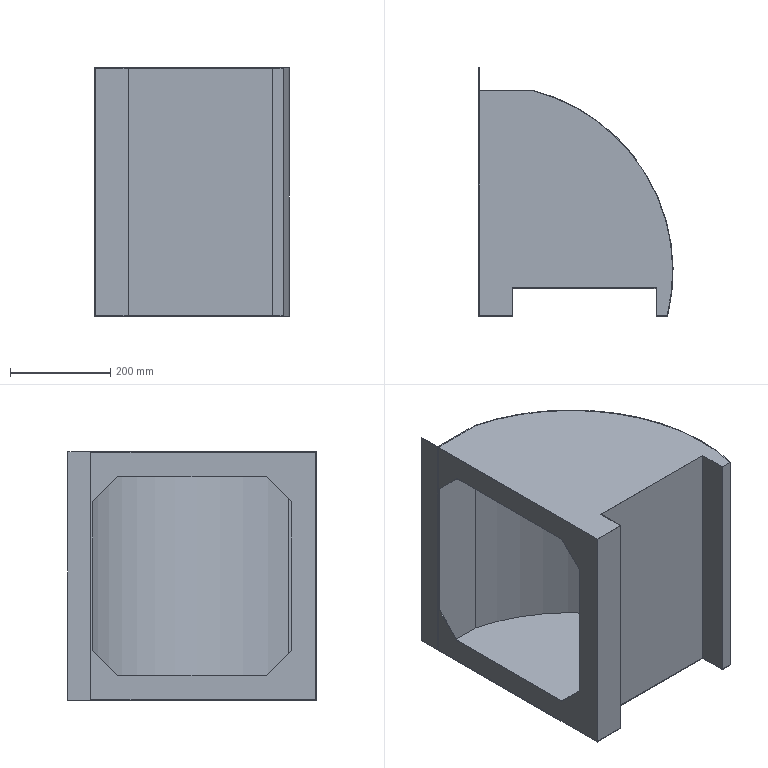Part | SolidWorks | features Extrusion 1, ICE 1, Shell 1 | 1 solid | 33 faces | box 386.98 x 495 x 495.029 mm | volume 841462 mm3 | plane 31 | cylinder 2 | commonest cylinder face diameters 740.359 x1 742.159 x1
STEP:
#1=CARTESIAN_POINT('',(0.,480.,495.));
#2=VERTEX_POINT('',#1);
#3=CARTESIAN_POINT('',(0.,480.,494.971));
#4=VERTEX_POINT('',#3);
#5=CARTESIAN_POINT('',(0.,480.,495.));
#6=DIRECTION('',(0.,0.,-1.));
#7=VECTOR('',#6,1000.);
#8=LINE('',#5,#7);
#9=EDGE_CURVE('',#2,#4,#8,.T.);
#10=ORIENTED_EDGE('',*,*,#9,.T.);
#11=CARTESIAN_POINT('',(0.,495.,494.971));
#12=VERTEX_POINT('',#11);
#13=CARTESIAN_POINT('',(0.,0.,494.971));
#14=DIRECTION('',(0.,1.,0.));
#15=VECTOR('',#14,1000.);
#16=LINE('',#13,#15);
#17=EDGE_CURVE('',#4,#12,#16,.T.);
#18=ORIENTED_EDGE('',*,*,#17,.T.);
#19=CARTESIAN_POINT('',(0.,495.,-0.02854));
#20=VERTEX_POINT('',#19);
#21=CARTESIAN_POINT('',(0.,495.,0.));
#22=DIRECTION('',(0.,0.,-1.));
#23=VECTOR('',#22,1000.);
#24=LINE('',#21,#23);
#25=EDGE_CURVE('',#12,#20,#24,.T.);
#26=ORIENTED_EDGE('',*,*,#25,.T.);
#27=CARTESIAN_POINT('',(0.,0.,-0.02854));
#28=VERTEX_POINT('',#27);
#29=CARTESIAN_POINT('',(0.,0.,-0.02854));
#30=DIRECTION('',(0.,-1.,0.));
#31=VECTOR('',#30,1000.);
#32=LINE('',#29,#31);
#33=EDGE_CURVE('',#20,#28,#32,.T.);
#34=ORIENTED_EDGE('',*,*,#33,.T.);
#35=CARTESIAN_POINT('',(0.,0.,495.));
#36=VERTEX_POINT('',#35);
#37=CARTESIAN_POINT('',(0.,0.,495.));
#38=DIRECTION('',(0.,0.,-1.));
#39=VECTOR('',#38,1000.);
#40=LINE('',#37,#39);
#41=EDGE_CURVE('',#36,#28,#40,.T.);
#42=ORIENTED_EDGE('',*,*,#41,.F.);
#43=CARTESIAN_POINT('',(0.,450.,495.));
#44=DIRECTION('',(0.,-1.,0.));
#45=VECTOR('',#44,1000.);
#46=LINE('',#43,#45);
#47=EDGE_CURVE('',#2,#36,#46,.T.);
#48=ORIENTED_EDGE('',*,*,#47,.F.);
#49=EDGE_LOOP('',(#10,#18,#26,#34,#42,#48));
#50=FACE_OUTER_BOUND('',#49,.T.);
#51=CARTESIAN_POINT('',(0.,50.,394.971));
#52=VERTEX_POINT('',#51);
#53=CARTESIAN_POINT('',(0.,100.,444.971));
#54=VERTEX_POINT('',#53);
#55=CARTESIAN_POINT('',(0.,-172.486,172.486));
#56=DIRECTION('',(0.,0.7071,0.7071));
#57=VECTOR('',#56,1000.);
#58=LINE('',#55,#57);
#59=EDGE_CURVE('',#52,#54,#58,.T.);
#60=ORIENTED_EDGE('',*,*,#59,.F.);
#61=CARTESIAN_POINT('',(0.,50.,99.971));
#62=VERTEX_POINT('',#61);
#63=CARTESIAN_POINT('',(0.,50.,0.));
#64=DIRECTION('',(0.,0.,1.));
#65=VECTOR('',#64,1000.);
#66=LINE('',#63,#65);
#67=EDGE_CURVE('',#62,#52,#66,.T.);
#68=ORIENTED_EDGE('',*,*,#67,.F.);
#69=CARTESIAN_POINT('',(0.,100.,49.971));
#70=VERTEX_POINT('',#69);
#71=CARTESIAN_POINT('',(0.,74.986,74.986));
#72=DIRECTION('',(0.,0.7071,-0.7071));
#73=VECTOR('',#72,1000.);
#74=LINE('',#71,#73);
#75=EDGE_CURVE('',#62,#70,#74,.T.);
#76=ORIENTED_EDGE('',*,*,#75,.T.);
#77=CARTESIAN_POINT('',(0.,395.,49.971));
#78=VERTEX_POINT('',#77);
#79=CARTESIAN_POINT('',(0.,0.,49.971));
#80=DIRECTION('',(0.,-1.,0.));
#81=VECTOR('',#80,1000.);
#82=LINE('',#79,#81);
#83=EDGE_CURVE('',#78,#70,#82,.T.);
#84=ORIENTED_EDGE('',*,*,#83,.F.);
#85=CARTESIAN_POINT('',(0.,445.,99.971));
#86=VERTEX_POINT('',#85);
#87=CARTESIAN_POINT('',(0.,172.514,-172.514));
#88=DIRECTION('',(0.,-0.7071,-0.7071));
#89=VECTOR('',#88,1000.);
#90=LINE('',#87,#89);
#91=EDGE_CURVE('',#86,#78,#90,.T.);
#92=ORIENTED_EDGE('',*,*,#91,.F.);
#93=CARTESIAN_POINT('',(0.,445.,394.971));
#94=VERTEX_POINT('',#93);
#95=CARTESIAN_POINT('',(0.,445.,0.));
#96=DIRECTION('',(0.,0.,-1.));
#97=VECTOR('',#96,1000.);
#98=LINE('',#95,#97);
#99=EDGE_CURVE('',#94,#86,#98,.T.);
#100=ORIENTED_EDGE('',*,*,#99,.F.);
#101=CARTESIAN_POINT('',(0.,395.,444.971));
#102=VERTEX_POINT('',#101);
#103=CARTESIAN_POINT('',(0.,419.986,419.986));
#104=DIRECTION('',(0.,-0.7071,0.7071));
#105=VECTOR('',#104,1000.);
#106=LINE('',#103,#105);
#107=EDGE_CURVE('',#94,#102,#106,.T.);
#108=ORIENTED_EDGE('',*,*,#107,.T.);
#109=CARTESIAN_POINT('',(0.,0.,444.971));
#110=DIRECTION('',(0.,1.,0.));
#111=VECTOR('',#110,1000.);
#112=LINE('',#109,#111);
#113=EDGE_CURVE('',#54,#102,#112,.T.);
#114=ORIENTED_EDGE('',*,*,#113,.F.);
#115=EDGE_LOOP('',(#60,#68,#76,#84,#92,#100,#108,#114));
#116=FACE_BOUND('',#115,.T.);
#117=CARTESIAN_POINT('',(0.,450.,495.));
#118=DIRECTION('',(1.,0.,0.));
#119=DIRECTION('',(0.,0.,-1.));
#120=AXIS2_PLACEMENT_3D('',#117,#118,#119);
#121=PLANE('',#120);
#122=ADVANCED_FACE('',(#50,#116),#121,.F.);
#123=ORIENTED_EDGE('',*,*,#41,.T.);
#124=CARTESIAN_POINT('',(0.9,0.,-0.02854));
#125=VERTEX_POINT('',#124);
#126=CARTESIAN_POINT('',(0.9,0.,-0.02854));
#127=DIRECTION('',(-1.,0.,0.));
#128=VECTOR('',#127,1000.);
#129=LINE('',#126,#128);
#130=EDGE_CURVE('',#125,#28,#129,.T.);
#131=ORIENTED_EDGE('',*,*,#130,.F.);
#132=CARTESIAN_POINT('',(0.9,0.,0.));
#133=VERTEX_POINT('',#132);
#134=CARTESIAN_POINT('',(0.9,0.,0.));
#135=DIRECTION('',(0.,0.,1.));
#136=VECTOR('',#135,1000.);
#137=LINE('',#134,#136);
#138=EDGE_CURVE('',#125,#133,#137,.T.);
#139=ORIENTED_EDGE('',*,*,#138,.T.);
#140=CARTESIAN_POINT('',(67.,0.,0.));
#141=VERTEX_POINT('',#140);
#142=CARTESIAN_POINT('',(0.,0.,0.));
#143=DIRECTION('',(1.,0.,0.));
#144=VECTOR('',#143,1000.);
#145=LINE('',#142,#144);
#146=EDGE_CURVE('',#133,#141,#145,.T.);
#147=ORIENTED_EDGE('',*,*,#146,.T.);
#148=CARTESIAN_POINT('',(67.,0.,495.));
#149=VERTEX_POINT('',#148);
#150=CARTESIAN_POINT('',(67.,0.,495.));
#151=DIRECTION('',(0.,0.,-1.));
#152=VECTOR('',#151,1000.);
#153=LINE('',#150,#152);
#154=EDGE_CURVE('',#149,#141,#153,.T.);
#155=ORIENTED_EDGE('',*,*,#154,.F.);
#156=CARTESIAN_POINT('',(0.,0.,495.));
#157=DIRECTION('',(1.,0.,0.));
#158=VECTOR('',#157,1000.);
#159=LINE('',#156,#158);
#160=EDGE_CURVE('',#36,#149,#159,.T.);
#161=ORIENTED_EDGE('',*,*,#160,.F.);
#162=EDGE_LOOP('',(#123,#131,#139,#147,#155,#161));
#163=FACE_OUTER_BOUND('',#162,.T.);
#164=CARTESIAN_POINT('',(0.,0.,495.));
#165=DIRECTION('',(0.,1.,0.));
#166=DIRECTION('',(0.,0.,1.));
#167=AXIS2_PLACEMENT_3D('',#164,#165,#166);
#168=PLANE('',#167);
#169=ADVANCED_FACE('',(#163),#168,.F.);
#170=CARTESIAN_POINT('',(67.,55.18,0.));
#171=VERTEX_POINT('',#170);
#172=CARTESIAN_POINT('',(67.,0.,0.));
#173=DIRECTION('',(0.,1.,0.));
#174=VECTOR('',#173,1000.);
#175=LINE('',#172,#174);
#176=EDGE_CURVE('',#141,#171,#175,.T.);
#177=ORIENTED_EDGE('',*,*,#176,.T.);
#178=CARTESIAN_POINT('',(67.,55.18,495.));
#179=VERTEX_POINT('',#178);
#180=CARTESIAN_POINT('',(67.,55.18,495.));
#181=DIRECTION('',(0.,0.,-1.));
#182=VECTOR('',#181,1000.);
#183=LINE('',#180,#182);
#184=EDGE_CURVE('',#179,#171,#183,.T.);
#185=ORIENTED_EDGE('',*,*,#184,.F.);
#186=CARTESIAN_POINT('',(67.,0.,495.));
#187=DIRECTION('',(0.,1.,0.));
#188=VECTOR('',#187,1000.);
#189=LINE('',#186,#188);
#190=EDGE_CURVE('',#149,#179,#189,.T.);
#191=ORIENTED_EDGE('',*,*,#190,.F.);
#192=ORIENTED_EDGE('',*,*,#154,.T.);
#193=EDGE_LOOP('',(#177,#185,#191,#192));
#194=FACE_OUTER_BOUND('',#193,.T.);
#195=CARTESIAN_POINT('',(67.,0.,495.));
#196=DIRECTION('',(-1.,0.,0.));
#197=DIRECTION('',(0.,0.,1.));
#198=AXIS2_PLACEMENT_3D('',#195,#196,#197);
#199=PLANE('',#198);
#200=ADVANCED_FACE('',(#194),#199,.F.);
#201=CARTESIAN_POINT('',(352.9,55.18,0.));
#202=VERTEX_POINT('',#201);
#203=CARTESIAN_POINT('',(67.,55.18,0.));
#204=DIRECTION('',(1.,0.,0.));
#205=VECTOR('',#204,1000.);
#206=LINE('',#203,#205);
#207=EDGE_CURVE('',#171,#202,#206,.T.);
#208=ORIENTED_EDGE('',*,*,#207,.T.);
#209=CARTESIAN_POINT('',(352.9,55.18,495.));
#210=VERTEX_POINT('',#209);
#211=CARTESIAN_POINT('',(352.9,55.18,495.));
#212=DIRECTION('',(0.,0.,-1.));
#213=VECTOR('',#212,1000.);
#214=LINE('',#211,#213);
#215=EDGE_CURVE('',#210,#202,#214,.T.);
#216=ORIENTED_EDGE('',*,*,#215,.F.);
#217=CARTESIAN_POINT('',(67.,55.18,495.));
#218=DIRECTION('',(1.,0.,0.));
#219=VECTOR('',#218,1000.);
#220=LINE('',#217,#219);
#221=EDGE_CURVE('',#179,#210,#220,.T.);
#222=ORIENTED_EDGE('',*,*,#221,.F.);
#223=ORIENTED_EDGE('',*,*,#184,.T.);
#224=EDGE_LOOP('',(#208,#216,#222,#223));
#225=FACE_OUTER_BOUND('',#224,.T.);
#226=CARTESIAN_POINT('',(67.,55.18,495.));
#227=DIRECTION('',(0.,1.,0.));
#228=DIRECTION('',(0.,0.,1.));
#229=AXIS2_PLACEMENT_3D('',#226,#227,#228);
#230=PLANE('',#229);
#231=ADVANCED_FACE('',(#225),#230,.F.);
#232=CARTESIAN_POINT('',(352.9,0.,0.));
#233=VERTEX_POINT('',#232);
#234=CARTESIAN_POINT('',(352.9,55.18,0.));
#235=DIRECTION('',(0.,-1.,0.));
#236=VECTOR('',#235,1000.);
#237=LINE('',#234,#236);
#238=EDGE_CURVE('',#202,#233,#237,.T.);
#239=ORIENTED_EDGE('',*,*,#238,.T.);
#240=CARTESIAN_POINT('',(352.9,0.,495.));
#241=VERTEX_POINT('',#240);
#242=CARTESIAN_POINT('',(352.9,0.,495.));
#243=DIRECTION('',(0.,0.,-1.));
#244=VECTOR('',#243,1000.);
#245=LINE('',#242,#244);
#246=EDGE_CURVE('',#241,#233,#245,.T.);
#247=ORIENTED_EDGE('',*,*,#246,.F.);
#248=CARTESIAN_POINT('',(352.9,55.18,495.));
#249=DIRECTION('',(0.,-1.,0.));
#250=VECTOR('',#249,1000.);
#251=LINE('',#248,#250);
#252=EDGE_CURVE('',#210,#241,#251,.T.);
#253=ORIENTED_EDGE('',*,*,#252,.F.);
#254=ORIENTED_EDGE('',*,*,#215,.T.);
#255=EDGE_LOOP('',(#239,#247,#253,#254));
#256=FACE_OUTER_BOUND('',#255,.T.);
#257=CARTESIAN_POINT('',(352.9,55.18,495.));
#258=DIRECTION('',(1.,0.,0.));
#259=DIRECTION('',(0.,0.,-1.));
#260=AXIS2_PLACEMENT_3D('',#257,#258,#259);
#261=PLANE('',#260);
#262=ADVANCED_FACE('',(#256),#261,.F.);
#263=CARTESIAN_POINT('',(375.9,0.,0.));
#264=VERTEX_POINT('',#263);
#265=CARTESIAN_POINT('',(352.9,0.,0.));
#266=DIRECTION('',(1.,0.,0.));
#267=VECTOR('',#266,1000.);
#268=LINE('',#265,#267);
#269=EDGE_CURVE('',#233,#264,#268,.T.);
#270=ORIENTED_EDGE('',*,*,#269,.T.);
#271=CARTESIAN_POINT('',(375.9,0.,495.));
#272=VERTEX_POINT('',#271);
#273=CARTESIAN_POINT('',(375.9,0.,495.));
#274=DIRECTION('',(0.,0.,-1.));
#275=VECTOR('',#274,1000.);
#276=LINE('',#273,#275);
#277=EDGE_CURVE('',#272,#264,#276,.T.);
#278=ORIENTED_EDGE('',*,*,#277,.F.);
#279=CARTESIAN_POINT('',(352.9,0.,495.));
#280=DIRECTION('',(1.,0.,0.));
#281=VECTOR('',#280,1000.);
#282=LINE('',#279,#281);
#283=EDGE_CURVE('',#241,#272,#282,.T.);
#284=ORIENTED_EDGE('',*,*,#283,.F.);
#285=ORIENTED_EDGE('',*,*,#246,.T.);
#286=EDGE_LOOP('',(#270,#278,#284,#285));
#287=FACE_OUTER_BOUND('',#286,.T.);
#288=CARTESIAN_POINT('',(352.9,0.,495.));
#289=DIRECTION('',(0.,1.,0.));
#290=DIRECTION('',(0.,0.,1.));
#291=AXIS2_PLACEMENT_3D('',#288,#289,#290);
#292=PLANE('',#291);
#293=ADVANCED_FACE('',(#287),#292,.F.);
#294=CARTESIAN_POINT('',(105.9,450.,0.));
#295=VERTEX_POINT('',#294);
#296=CARTESIAN_POINT('',(15.9,90.,0.));
#297=DIRECTION('',(0.,0.,1.));
#298=DIRECTION('',(-1.,0.,0.));
#299=AXIS2_PLACEMENT_3D('',#296,#297,#298);
#300=CIRCLE('',#299,371.08);
#301=EDGE_CURVE('',#264,#295,#300,.T.);
#302=ORIENTED_EDGE('',*,*,#301,.T.);
#303=CARTESIAN_POINT('',(105.9,450.,495.));
#304=VERTEX_POINT('',#303);
#305=CARTESIAN_POINT('',(105.9,450.,495.));
#306=DIRECTION('',(0.,0.,-1.));
#307=VECTOR('',#306,1000.);
#308=LINE('',#305,#307);
#309=EDGE_CURVE('',#304,#295,#308,.T.);
#310=ORIENTED_EDGE('',*,*,#309,.F.);
#311=CARTESIAN_POINT('',(15.9,90.,495.));
#312=DIRECTION('',(0.,0.,1.));
#313=DIRECTION('',(-1.,0.,0.));
#314=AXIS2_PLACEMENT_3D('',#311,#312,#313);
#315=CIRCLE('',#314,371.08);
#316=EDGE_CURVE('',#272,#304,#315,.T.);
#317=ORIENTED_EDGE('',*,*,#316,.F.);
#318=ORIENTED_EDGE('',*,*,#277,.T.);
#319=EDGE_LOOP('',(#302,#310,#317,#318));
#320=FACE_OUTER_BOUND('',#319,.T.);
#321=CARTESIAN_POINT('',(15.9,90.,495.));
#322=DIRECTION('',(0.,0.,-1.));
#323=DIRECTION('',(-1.,0.,0.));
#324=AXIS2_PLACEMENT_3D('',#321,#322,#323);
#325=CYLINDRICAL_SURFACE('',#324,371.08);
#326=ADVANCED_FACE('',(#320),#325,.T.);
#327=CARTESIAN_POINT('',(0.9,450.,0.));
#328=VERTEX_POINT('',#327);
#329=CARTESIAN_POINT('',(0.9,450.,0.));
#330=DIRECTION('',(-1.,0.,0.));
#331=VECTOR('',#330,1000.);
#332=LINE('',#329,#331);
#333=EDGE_CURVE('',#295,#328,#332,.T.);
#334=ORIENTED_EDGE('',*,*,#333,.T.);
#335=CARTESIAN_POINT('',(0.9,450.,495.));
#336=VERTEX_POINT('',#335);
#337=CARTESIAN_POINT('',(0.9,450.,495.));
#338=DIRECTION('',(0.,0.,-1.));
#339=VECTOR('',#338,1000.);
#340=LINE('',#337,#339);
#341=EDGE_CURVE('',#336,#328,#340,.T.);
#342=ORIENTED_EDGE('',*,*,#341,.F.);
#343=CARTESIAN_POINT('',(0.9,450.,495.));
#344=DIRECTION('',(-1.,0.,0.));
#345=VECTOR('',#344,1000.);
#346=LINE('',#343,#345);
#347=EDGE_CURVE('',#304,#336,#346,.T.);
#348=ORIENTED_EDGE('',*,*,#347,.F.);
#349=ORIENTED_EDGE('',*,*,#309,.T.);
#350=EDGE_LOOP('',(#334,#342,#348,#349));
#351=FACE_OUTER_BOUND('',#350,.T.);
#352=CARTESIAN_POINT('',(0.9,450.,495.));
#353=DIRECTION('',(0.,-1.,0.));
#354=DIRECTION('',(0.,0.,-1.));
#355=AXIS2_PLACEMENT_3D('',#352,#353,#354);
#356=PLANE('',#355);
#357=ADVANCED_FACE('',(#351),#356,.F.);
#358=ORIENTED_EDGE('',*,*,#341,.T.);
#359=CARTESIAN_POINT('',(0.9,90.,0.));
#360=DIRECTION('',(0.,-1.,0.));
#361=VECTOR('',#360,1000.);
#362=LINE('',#359,#361);
#363=EDGE_CURVE('',#328,#133,#362,.T.);
#364=ORIENTED_EDGE('',*,*,#363,.T.);
#365=ORIENTED_EDGE('',*,*,#138,.F.);
#366=CARTESIAN_POINT('',(0.9,495.,-0.02854));
#367=VERTEX_POINT('',#366);
#368=CARTESIAN_POINT('',(0.9,0.,-0.02854));
#369=DIRECTION('',(0.,-1.,0.));
#370=VECTOR('',#369,1000.);
#371=LINE('',#368,#370);
#372=EDGE_CURVE('',#367,#125,#371,.T.);
#373=ORIENTED_EDGE('',*,*,#372,.F.);
#374=CARTESIAN_POINT('',(0.9,495.,494.971));
#375=VERTEX_POINT('',#374);
#376=CARTESIAN_POINT('',(0.9,495.,0.));
#377=DIRECTION('',(0.,0.,-1.));
#378=VECTOR('',#377,1000.);
#379=LINE('',#376,#378);
#380=EDGE_CURVE('',#375,#367,#379,.T.);
#381=ORIENTED_EDGE('',*,*,#380,.F.);
#382=CARTESIAN_POINT('',(0.9,480.,494.971));
#383=VERTEX_POINT('',#382);
#384=CARTESIAN_POINT('',(0.9,0.,494.971));
#385=DIRECTION('',(0.,1.,0.));
#386=VECTOR('',#385,1000.);
#387=LINE('',#384,#386);
#388=EDGE_CURVE('',#383,#375,#387,.T.);
#389=ORIENTED_EDGE('',*,*,#388,.F.);
#390=CARTESIAN_POINT('',(0.9,480.,495.));
#391=VERTEX_POINT('',#390);
#392=CARTESIAN_POINT('',(0.9,480.,495.));
#393=DIRECTION('',(0.,0.,-1.));
#394=VECTOR('',#393,1000.);
#395=LINE('',#392,#394);
#396=EDGE_CURVE('',#391,#383,#395,.T.);
#397=ORIENTED_EDGE('',*,*,#396,.F.);
#398=CARTESIAN_POINT('',(0.9,480.,495.));
#399=DIRECTION('',(0.,1.,0.));
#400=VECTOR('',#399,1000.);
#401=LINE('',#398,#400);
#402=EDGE_CURVE('',#336,#391,#401,.T.);
#403=ORIENTED_EDGE('',*,*,#402,.F.);
#404=EDGE_LOOP('',(#358,#364,#365,#373,#381,#389,#397,#403));
#405=FACE_OUTER_BOUND('',#404,.T.);
#406=CARTESIAN_POINT('',(0.9,480.,495.));
#407=DIRECTION('',(-1.,0.,0.));
#408=DIRECTION('',(0.,-1.,0.));
#409=AXIS2_PLACEMENT_3D('',#406,#407,#408);
#410=PLANE('',#409);
#411=ADVANCED_FACE('',(#405),#410,.F.);
#412=ORIENTED_EDGE('',*,*,#396,.T.);
#413=CARTESIAN_POINT('',(0.,480.,494.971));
#414=DIRECTION('',(-1.,0.,0.));
#415=VECTOR('',#414,1000.);
#416=LINE('',#413,#415);
#417=EDGE_CURVE('',#383,#4,#416,.T.);
#418=ORIENTED_EDGE('',*,*,#417,.T.);
#419=ORIENTED_EDGE('',*,*,#9,.F.);
#420=CARTESIAN_POINT('',(0.,480.,495.));
#421=DIRECTION('',(-1.,0.,0.));
#422=VECTOR('',#421,1000.);
#423=LINE('',#420,#422);
#424=EDGE_CURVE('',#391,#2,#423,.T.);
#425=ORIENTED_EDGE('',*,*,#424,.F.);
#426=EDGE_LOOP('',(#412,#418,#419,#425));
#427=FACE_OUTER_BOUND('',#426,.T.);
#428=CARTESIAN_POINT('',(0.,480.,495.));
#429=DIRECTION('',(0.,-1.,0.));
#430=DIRECTION('',(0.,0.,-1.));
#431=AXIS2_PLACEMENT_3D('',#428,#429,#430);
#432=PLANE('',#431);
#433=ADVANCED_FACE('',(#427),#432,.F.);
#434=ORIENTED_EDGE('',*,*,#47,.T.);
#435=ORIENTED_EDGE('',*,*,#160,.T.);
#436=ORIENTED_EDGE('',*,*,#190,.T.);
#437=ORIENTED_EDGE('',*,*,#221,.T.);
#438=ORIENTED_EDGE('',*,*,#252,.T.);
#439=ORIENTED_EDGE('',*,*,#283,.T.);
#440=ORIENTED_EDGE('',*,*,#316,.T.);
#441=ORIENTED_EDGE('',*,*,#347,.T.);
#442=ORIENTED_EDGE('',*,*,#402,.T.);
#443=ORIENTED_EDGE('',*,*,#424,.T.);
#444=EDGE_LOOP('',(#434,#435,#436,#437,#438,#439,#440,#441,#442,#443));
#445=FACE_OUTER_BOUND('',#444,.T.);
#446=CARTESIAN_POINT('',(15.9,90.,495.));
#447=DIRECTION('',(0.,0.,-1.));
#448=DIRECTION('',(-1.,0.,0.));
#449=AXIS2_PLACEMENT_3D('',#446,#447,#448);
#450=PLANE('',#449);
#451=ADVANCED_FACE('',(#445),#450,.F.);
#452=ORIENTED_EDGE('',*,*,#363,.F.);
#453=ORIENTED_EDGE('',*,*,#333,.F.);
#454=ORIENTED_EDGE('',*,*,#301,.F.);
#455=ORIENTED_EDGE('',*,*,#269,.F.);
#456=ORIENTED_EDGE('',*,*,#238,.F.);
#457=ORIENTED_EDGE('',*,*,#207,.F.);
#458=ORIENTED_EDGE('',*,*,#176,.F.);
#459=ORIENTED_EDGE('',*,*,#146,.F.);
#460=EDGE_LOOP('',(#452,#453,#454,#455,#456,#457,#458,#459));
#461=FACE_OUTER_BOUND('',#460,.T.);
#462=CARTESIAN_POINT('',(15.9,90.,0.));
#463=DIRECTION('',(0.,0.,-1.));
#464=DIRECTION('',(-1.,0.,0.));
#465=AXIS2_PLACEMENT_3D('',#462,#463,#464);
#466=PLANE('',#465);
#467=ADVANCED_FACE('',(#461),#466,.T.);
#468=ORIENTED_EDGE('',*,*,#113,.T.);
#469=CARTESIAN_POINT('',(0.9,395.,444.971));
#470=VERTEX_POINT('',#469);
#471=CARTESIAN_POINT('',(0.9,395.,444.971));
#472=DIRECTION('',(-1.,0.,0.));
#473=VECTOR('',#472,1000.);
#474=LINE('',#471,#473);
#475=EDGE_CURVE('',#470,#102,#474,.T.);
#476=ORIENTED_EDGE('',*,*,#475,.F.);
#477=CARTESIAN_POINT('',(0.9,100.,444.971));
#478=VERTEX_POINT('',#477);
#479=CARTESIAN_POINT('',(0.9,0.,444.971));
#480=DIRECTION('',(0.,1.,0.));
#481=VECTOR('',#480,1000.);
#482=LINE('',#479,#481);
#483=EDGE_CURVE('',#478,#470,#482,.T.);
#484=ORIENTED_EDGE('',*,*,#483,.F.);
#485=CARTESIAN_POINT('',(0.9,100.,444.971));
#486=DIRECTION('',(-1.,0.,0.));
#487=VECTOR('',#486,1000.);
#488=LINE('',#485,#487);
#489=EDGE_CURVE('',#478,#54,#488,.T.);
#490=ORIENTED_EDGE('',*,*,#489,.T.);
#491=EDGE_LOOP('',(#468,#476,#484,#490));
#492=FACE_OUTER_BOUND('',#491,.T.);
#493=CARTESIAN_POINT('',(0.9,0.,444.971));
#494=DIRECTION('',(0.,0.,1.));
#495=DIRECTION('',(1.,0.,0.));
#496=AXIS2_PLACEMENT_3D('',#493,#494,#495);
#497=PLANE('',#496);
#498=ADVANCED_FACE('',(#492),#497,.F.);
#499=ORIENTED_EDGE('',*,*,#107,.F.);
#500=CARTESIAN_POINT('',(0.9,445.,394.971));
#501=VERTEX_POINT('',#500);
#502=CARTESIAN_POINT('',(0.9,445.,394.971));
#503=DIRECTION('',(-1.,0.,0.));
#504=VECTOR('',#503,1000.);
#505=LINE('',#502,#504);
#506=EDGE_CURVE('',#501,#94,#505,.T.);
#507=ORIENTED_EDGE('',*,*,#506,.F.);
#508=CARTESIAN_POINT('',(0.9,419.986,419.986));
#509=DIRECTION('',(0.,-0.7071,0.7071));
#510=VECTOR('',#509,1000.);
#511=LINE('',#508,#510);
#512=EDGE_CURVE('',#501,#470,#511,.T.);
#513=ORIENTED_EDGE('',*,*,#512,.T.);
#514=ORIENTED_EDGE('',*,*,#475,.T.);
#515=EDGE_LOOP('',(#499,#507,#513,#514));
#516=FACE_OUTER_BOUND('',#515,.T.);
#517=CARTESIAN_POINT('',(0.9,419.986,419.986));
#518=DIRECTION('',(0.,-0.7071,-0.7071));
#519=DIRECTION('',(0.,0.7071,-0.7071));
#520=AXIS2_PLACEMENT_3D('',#517,#518,#519);
#521=PLANE('',#520);
#522=ADVANCED_FACE('',(#516),#521,.T.);
#523=ORIENTED_EDGE('',*,*,#99,.T.);
#524=CARTESIAN_POINT('',(0.9,445.,99.971));
#525=VERTEX_POINT('',#524);
#526=CARTESIAN_POINT('',(0.9,445.,99.971));
#527=DIRECTION('',(-1.,0.,0.));
#528=VECTOR('',#527,1000.);
#529=LINE('',#526,#528);
#530=EDGE_CURVE('',#525,#86,#529,.T.);
#531=ORIENTED_EDGE('',*,*,#530,.F.);
#532=CARTESIAN_POINT('',(0.9,445.,0.));
#533=DIRECTION('',(0.,0.,-1.));
#534=VECTOR('',#533,1000.);
#535=LINE('',#532,#534);
#536=EDGE_CURVE('',#501,#525,#535,.T.);
#537=ORIENTED_EDGE('',*,*,#536,.F.);
#538=ORIENTED_EDGE('',*,*,#506,.T.);
#539=EDGE_LOOP('',(#523,#531,#537,#538));
#540=FACE_OUTER_BOUND('',#539,.T.);
#541=CARTESIAN_POINT('',(0.9,445.,0.));
#542=DIRECTION('',(0.,1.,0.));
#543=DIRECTION('',(0.,0.,1.));
#544=AXIS2_PLACEMENT_3D('',#541,#542,#543);
#545=PLANE('',#544);
#546=ADVANCED_FACE('',(#540),#545,.F.);
#547=ORIENTED_EDGE('',*,*,#91,.T.);
#548=CARTESIAN_POINT('',(0.9,395.,49.971));
#549=VERTEX_POINT('',#548);
#550=CARTESIAN_POINT('',(0.9,395.,49.971));
#551=DIRECTION('',(-1.,0.,0.));
#552=VECTOR('',#551,1000.);
#553=LINE('',#550,#552);
#554=EDGE_CURVE('',#549,#78,#553,.T.);
#555=ORIENTED_EDGE('',*,*,#554,.F.);
#556=CARTESIAN_POINT('',(0.9,172.514,-172.514));
#557=DIRECTION('',(0.,-0.7071,-0.7071));
#558=VECTOR('',#557,1000.);
#559=LINE('',#556,#558);
#560=EDGE_CURVE('',#525,#549,#559,.T.);
#561=ORIENTED_EDGE('',*,*,#560,.F.);
#562=ORIENTED_EDGE('',*,*,#530,.T.);
#563=EDGE_LOOP('',(#547,#555,#561,#562));
#564=FACE_OUTER_BOUND('',#563,.T.);
#565=CARTESIAN_POINT('',(0.9,172.514,-172.514));
#566=DIRECTION('',(0.,0.7071,-0.7071));
#567=DIRECTION('',(0.,0.7071,0.7071));
#568=AXIS2_PLACEMENT_3D('',#565,#566,#567);
#569=PLANE('',#568);
#570=ADVANCED_FACE('',(#564),#569,.F.);
#571=ORIENTED_EDGE('',*,*,#83,.T.);
#572=CARTESIAN_POINT('',(0.9,100.,49.971));
#573=VERTEX_POINT('',#572);
#574=CARTESIAN_POINT('',(0.9,100.,49.971));
#575=DIRECTION('',(-1.,0.,0.));
#576=VECTOR('',#575,1000.);
#577=LINE('',#574,#576);
#578=EDGE_CURVE('',#573,#70,#577,.T.);
#579=ORIENTED_EDGE('',*,*,#578,.F.);
#580=CARTESIAN_POINT('',(0.9,0.,49.971));
#581=DIRECTION('',(0.,-1.,0.));
#582=VECTOR('',#581,1000.);
#583=LINE('',#580,#582);
#584=EDGE_CURVE('',#549,#573,#583,.T.);
#585=ORIENTED_EDGE('',*,*,#584,.F.);
#586=ORIENTED_EDGE('',*,*,#554,.T.);
#587=EDGE_LOOP('',(#571,#579,#585,#586));
#588=FACE_OUTER_BOUND('',#587,.T.);
#589=CARTESIAN_POINT('',(0.9,0.,49.971));
#590=DIRECTION('',(0.,0.,-1.));
#591=DIRECTION('',(-1.,0.,0.));
#592=AXIS2_PLACEMENT_3D('',#589,#590,#591);
#593=PLANE('',#592);
#594=ADVANCED_FACE('',(#588),#593,.F.);
#595=ORIENTED_EDGE('',*,*,#75,.F.);
#596=CARTESIAN_POINT('',(0.9,50.,99.971));
#597=VERTEX_POINT('',#596);
#598=CARTESIAN_POINT('',(0.9,50.,99.971));
#599=DIRECTION('',(-1.,0.,0.));
#600=VECTOR('',#599,1000.);
#601=LINE('',#598,#600);
#602=EDGE_CURVE('',#597,#62,#601,.T.);
#603=ORIENTED_EDGE('',*,*,#602,.F.);
#604=CARTESIAN_POINT('',(0.9,74.986,74.986));
#605=DIRECTION('',(0.,0.7071,-0.7071));
#606=VECTOR('',#605,1000.);
#607=LINE('',#604,#606);
#608=EDGE_CURVE('',#597,#573,#607,.T.);
#609=ORIENTED_EDGE('',*,*,#608,.T.);
#610=ORIENTED_EDGE('',*,*,#578,.T.);
#611=EDGE_LOOP('',(#595,#603,#609,#610));
#612=FACE_OUTER_BOUND('',#611,.T.);
#613=CARTESIAN_POINT('',(0.9,74.986,74.986));
#614=DIRECTION('',(0.,0.7071,0.7071));
#615=DIRECTION('',(0.,-0.7071,0.7071));
#616=AXIS2_PLACEMENT_3D('',#613,#614,#615);
#617=PLANE('',#616);
#618=ADVANCED_FACE('',(#612),#617,.T.);
#619=ORIENTED_EDGE('',*,*,#67,.T.);
#620=CARTESIAN_POINT('',(0.9,50.,394.971));
#621=VERTEX_POINT('',#620);
#622=CARTESIAN_POINT('',(0.9,50.,394.971));
#623=DIRECTION('',(-1.,0.,0.));
#624=VECTOR('',#623,1000.);
#625=LINE('',#622,#624);
#626=EDGE_CURVE('',#621,#52,#625,.T.);
#627=ORIENTED_EDGE('',*,*,#626,.F.);
#628=CARTESIAN_POINT('',(0.9,50.,0.));
#629=DIRECTION('',(0.,0.,1.));
#630=VECTOR('',#629,1000.);
#631=LINE('',#628,#630);
#632=EDGE_CURVE('',#597,#621,#631,.T.);
#633=ORIENTED_EDGE('',*,*,#632,.F.);
#634=ORIENTED_EDGE('',*,*,#602,.T.);
#635=EDGE_LOOP('',(#619,#627,#633,#634));
#636=FACE_OUTER_BOUND('',#635,.T.);
#637=CARTESIAN_POINT('',(0.9,50.,0.));
#638=DIRECTION('',(0.,-1.,0.));
#639=DIRECTION('',(0.,0.,-1.));
#640=AXIS2_PLACEMENT_3D('',#637,#638,#639);
#641=PLANE('',#640);
#642=ADVANCED_FACE('',(#636),#641,.F.);
#643=CARTESIAN_POINT('',(0.9,449.1,0.9));
#644=VERTEX_POINT('',#643);
#645=CARTESIAN_POINT('',(0.9,449.1,494.1));
#646=VERTEX_POINT('',#645);
#647=CARTESIAN_POINT('',(0.9,449.1,495.));
#648=DIRECTION('',(0.,0.,1.));
#649=VECTOR('',#648,1000.);
#650=LINE('',#647,#649);
#651=EDGE_CURVE('',#644,#646,#650,.T.);
#652=ORIENTED_EDGE('',*,*,#651,.T.);
#653=CARTESIAN_POINT('',(0.9,0.9,494.1));
#654=VERTEX_POINT('',#653);
#655=CARTESIAN_POINT('',(0.9,90.,494.1));
#656=DIRECTION('',(0.,-1.,0.));
#657=VECTOR('',#656,1000.);
#658=LINE('',#655,#657);
#659=EDGE_CURVE('',#646,#654,#658,.T.);
#660=ORIENTED_EDGE('',*,*,#659,.T.);
#661=CARTESIAN_POINT('',(0.9,0.9,0.9));
#662=VERTEX_POINT('',#661);
#663=CARTESIAN_POINT('',(0.9,0.9,495.));
#664=DIRECTION('',(0.,0.,-1.));
#665=VECTOR('',#664,1000.);
#666=LINE('',#663,#665);
#667=EDGE_CURVE('',#654,#662,#666,.T.);
#668=ORIENTED_EDGE('',*,*,#667,.T.);
#669=CARTESIAN_POINT('',(0.9,90.,0.9));
#670=DIRECTION('',(0.,-1.,0.));
#671=VECTOR('',#670,1000.);
#672=LINE('',#669,#671);
#673=EDGE_CURVE('',#644,#662,#672,.T.);
#674=ORIENTED_EDGE('',*,*,#673,.F.);
#675=EDGE_LOOP('',(#652,#660,#668,#674));
#676=FACE_OUTER_BOUND('',#675,.T.);
#677=CARTESIAN_POINT('',(0.9,-172.486,172.486));
#678=DIRECTION('',(0.,0.7071,0.7071));
#679=VECTOR('',#678,1000.);
#680=LINE('',#677,#679);
#681=EDGE_CURVE('',#621,#478,#680,.T.);
#682=ORIENTED_EDGE('',*,*,#681,.T.);
#683=ORIENTED_EDGE('',*,*,#483,.T.);
#684=ORIENTED_EDGE('',*,*,#512,.F.);
#685=ORIENTED_EDGE('',*,*,#536,.T.);
#686=ORIENTED_EDGE('',*,*,#560,.T.);
#687=ORIENTED_EDGE('',*,*,#584,.T.);
#688=ORIENTED_EDGE('',*,*,#608,.F.);
#689=ORIENTED_EDGE('',*,*,#632,.T.);
#690=EDGE_LOOP('',(#682,#683,#684,#685,#686,#687,#688,#689));
#691=FACE_BOUND('',#690,.T.);
#692=CARTESIAN_POINT('',(0.9,0.,0.));
#693=DIRECTION('',(1.,0.,0.));
#694=DIRECTION('',(0.,0.,-1.));
#695=AXIS2_PLACEMENT_3D('',#692,#693,#694);
#696=PLANE('',#695);
#697=ADVANCED_FACE('',(#676,#691),#696,.T.);
#698=ORIENTED_EDGE('',*,*,#59,.T.);
#699=ORIENTED_EDGE('',*,*,#489,.F.);
#700=ORIENTED_EDGE('',*,*,#681,.F.);
#701=ORIENTED_EDGE('',*,*,#626,.T.);
#702=EDGE_LOOP('',(#698,#699,#700,#701));
#703=FACE_OUTER_BOUND('',#702,.T.);
#704=CARTESIAN_POINT('',(0.9,-172.486,172.486));
#705=DIRECTION('',(0.,-0.7071,0.7071));
#706=DIRECTION('',(0.,-0.7071,-0.7071));
#707=AXIS2_PLACEMENT_3D('',#704,#705,#706);
#708=PLANE('',#707);
#709=ADVANCED_FACE('',(#703),#708,.F.);
#710=CARTESIAN_POINT('',(375.197,0.9,0.9));
#711=VERTEX_POINT('',#710);
#712=CARTESIAN_POINT('',(105.789,449.1,0.9));
#713=VERTEX_POINT('',#712);
#714=CARTESIAN_POINT('',(15.9,90.,0.9));
#715=DIRECTION('',(0.,0.,1.));
#716=DIRECTION('',(-1.,0.,0.));
#717=AXIS2_PLACEMENT_3D('',#714,#715,#716);
#718=CIRCLE('',#717,370.18);
#719=EDGE_CURVE('',#711,#713,#718,.T.);
#720=ORIENTED_EDGE('',*,*,#719,.F.);
#721=CARTESIAN_POINT('',(375.197,0.9,494.1));
#722=VERTEX_POINT('',#721);
#723=CARTESIAN_POINT('',(375.197,0.9,494.1));
#724=DIRECTION('',(0.,0.,-1.));
#725=VECTOR('',#724,1000.);
#726=LINE('',#723,#725);
#727=EDGE_CURVE('',#722,#711,#726,.T.);
#728=ORIENTED_EDGE('',*,*,#727,.F.);
#729=CARTESIAN_POINT('',(105.789,449.1,494.1));
#730=VERTEX_POINT('',#729);
#731=CARTESIAN_POINT('',(15.9,90.,494.1));
#732=DIRECTION('',(0.,0.,1.));
#733=DIRECTION('',(-1.,0.,0.));
#734=AXIS2_PLACEMENT_3D('',#731,#732,#733);
#735=CIRCLE('',#734,370.18);
#736=EDGE_CURVE('',#722,#730,#735,.T.);
#737=ORIENTED_EDGE('',*,*,#736,.T.);
#738=CARTESIAN_POINT('',(105.789,449.1,494.1));
#739=DIRECTION('',(0.,0.,-1.));
#740=VECTOR('',#739,1000.);
#741=LINE('',#738,#740);
#742=EDGE_CURVE('',#730,#713,#741,.T.);
#743=ORIENTED_EDGE('',*,*,#742,.T.);
#744=EDGE_LOOP('',(#720,#728,#737,#743));
#745=FACE_OUTER_BOUND('',#744,.T.);
#746=CARTESIAN_POINT('',(15.9,90.,495.));
#747=DIRECTION('',(0.,0.,-1.));
#748=DIRECTION('',(-1.,0.,0.));
#749=AXIS2_PLACEMENT_3D('',#746,#747,#748);
#750=CYLINDRICAL_SURFACE('',#749,370.18);
#751=ADVANCED_FACE('',(#745),#750,.F.);
#752=CARTESIAN_POINT('',(353.8,0.9,0.9));
#753=VERTEX_POINT('',#752);
#754=CARTESIAN_POINT('',(15.9,0.9,0.9));
#755=DIRECTION('',(1.,0.,0.));
#756=VECTOR('',#755,1000.);
#757=LINE('',#754,#756);
#758=EDGE_CURVE('',#753,#711,#757,.T.);
#759=ORIENTED_EDGE('',*,*,#758,.F.);
#760=CARTESIAN_POINT('',(353.8,0.9,494.1));
#761=VERTEX_POINT('',#760);
#762=CARTESIAN_POINT('',(353.8,0.9,495.));
#763=DIRECTION('',(0.,0.,-1.));
#764=VECTOR('',#763,1000.);
#765=LINE('',#762,#764);
#766=EDGE_CURVE('',#761,#753,#765,.T.);
#767=ORIENTED_EDGE('',*,*,#766,.F.);
#768=CARTESIAN_POINT('',(15.9,0.9,494.1));
#769=DIRECTION('',(1.,0.,0.));
#770=VECTOR('',#769,1000.);
#771=LINE('',#768,#770);
#772=EDGE_CURVE('',#761,#722,#771,.T.);
#773=ORIENTED_EDGE('',*,*,#772,.T.);
#774=ORIENTED_EDGE('',*,*,#727,.T.);
#775=EDGE_LOOP('',(#759,#767,#773,#774));
#776=FACE_OUTER_BOUND('',#775,.T.);
#777=CARTESIAN_POINT('',(352.9,0.9,495.));
#778=DIRECTION('',(0.,1.,0.));
#779=DIRECTION('',(0.,0.,1.));
#780=AXIS2_PLACEMENT_3D('',#777,#778,#779);
#781=PLANE('',#780);
#782=ADVANCED_FACE('',(#776),#781,.T.);
#783=CARTESIAN_POINT('',(353.8,56.08,0.9));
#784=VERTEX_POINT('',#783);
#785=CARTESIAN_POINT('',(353.8,90.,0.9));
#786=DIRECTION('',(0.,-1.,0.));
#787=VECTOR('',#786,1000.);
#788=LINE('',#785,#787);
#789=EDGE_CURVE('',#784,#753,#788,.T.);
#790=ORIENTED_EDGE('',*,*,#789,.F.);
#791=CARTESIAN_POINT('',(353.8,56.08,494.1));
#792=VERTEX_POINT('',#791);
#793=CARTESIAN_POINT('',(353.8,56.08,495.));
#794=DIRECTION('',(0.,0.,-1.));
#795=VECTOR('',#794,1000.);
#796=LINE('',#793,#795);
#797=EDGE_CURVE('',#792,#784,#796,.T.);
#798=ORIENTED_EDGE('',*,*,#797,.F.);
#799=CARTESIAN_POINT('',(353.8,90.,494.1));
#800=DIRECTION('',(0.,-1.,0.));
#801=VECTOR('',#800,1000.);
#802=LINE('',#799,#801);
#803=EDGE_CURVE('',#792,#761,#802,.T.);
#804=ORIENTED_EDGE('',*,*,#803,.T.);
#805=ORIENTED_EDGE('',*,*,#766,.T.);
#806=EDGE_LOOP('',(#790,#798,#804,#805));
#807=FACE_OUTER_BOUND('',#806,.T.);
#808=CARTESIAN_POINT('',(353.8,55.18,495.));
#809=DIRECTION('',(1.,0.,0.));
#810=DIRECTION('',(0.,0.,-1.));
#811=AXIS2_PLACEMENT_3D('',#808,#809,#810);
#812=PLANE('',#811);
#813=ADVANCED_FACE('',(#807),#812,.T.);
#814=CARTESIAN_POINT('',(66.1,56.08,0.9));
#815=VERTEX_POINT('',#814);
#816=CARTESIAN_POINT('',(15.9,56.08,0.9));
#817=DIRECTION('',(1.,0.,0.));
#818=VECTOR('',#817,1000.);
#819=LINE('',#816,#818);
#820=EDGE_CURVE('',#815,#784,#819,.T.);
#821=ORIENTED_EDGE('',*,*,#820,.F.);
#822=CARTESIAN_POINT('',(66.1,56.08,494.1));
#823=VERTEX_POINT('',#822);
#824=CARTESIAN_POINT('',(66.1,56.08,495.));
#825=DIRECTION('',(0.,0.,-1.));
#826=VECTOR('',#825,1000.);
#827=LINE('',#824,#826);
#828=EDGE_CURVE('',#823,#815,#827,.T.);
#829=ORIENTED_EDGE('',*,*,#828,.F.);
#830=CARTESIAN_POINT('',(15.9,56.08,494.1));
#831=DIRECTION('',(1.,0.,0.));
#832=VECTOR('',#831,1000.);
#833=LINE('',#830,#832);
#834=EDGE_CURVE('',#823,#792,#833,.T.);
#835=ORIENTED_EDGE('',*,*,#834,.T.);
#836=ORIENTED_EDGE('',*,*,#797,.T.);
#837=EDGE_LOOP('',(#821,#829,#835,#836));
#838=FACE_OUTER_BOUND('',#837,.T.);
#839=CARTESIAN_POINT('',(67.,56.08,495.));
#840=DIRECTION('',(0.,1.,0.));
#841=DIRECTION('',(0.,0.,1.));
#842=AXIS2_PLACEMENT_3D('',#839,#840,#841);
#843=PLANE('',#842);
#844=ADVANCED_FACE('',(#838),#843,.T.);
#845=CARTESIAN_POINT('',(66.1,0.9,0.9));
#846=VERTEX_POINT('',#845);
#847=CARTESIAN_POINT('',(66.1,90.,0.9));
#848=DIRECTION('',(0.,1.,0.));
#849=VECTOR('',#848,1000.);
#850=LINE('',#847,#849);
#851=EDGE_CURVE('',#846,#815,#850,.T.);
#852=ORIENTED_EDGE('',*,*,#851,.F.);
#853=CARTESIAN_POINT('',(66.1,0.9,494.1));
#854=VERTEX_POINT('',#853);
#855=CARTESIAN_POINT('',(66.1,0.9,495.));
#856=DIRECTION('',(0.,0.,-1.));
#857=VECTOR('',#856,1000.);
#858=LINE('',#855,#857);
#859=EDGE_CURVE('',#854,#846,#858,.T.);
#860=ORIENTED_EDGE('',*,*,#859,.F.);
#861=CARTESIAN_POINT('',(66.1,90.,494.1));
#862=DIRECTION('',(0.,1.,0.));
#863=VECTOR('',#862,1000.);
#864=LINE('',#861,#863);
#865=EDGE_CURVE('',#854,#823,#864,.T.);
#866=ORIENTED_EDGE('',*,*,#865,.T.);
#867=ORIENTED_EDGE('',*,*,#828,.T.);
#868=EDGE_LOOP('',(#852,#860,#866,#867));
#869=FACE_OUTER_BOUND('',#868,.T.);
#870=CARTESIAN_POINT('',(66.1,0.,495.));
#871=DIRECTION('',(-1.,0.,0.));
#872=DIRECTION('',(0.,0.,1.));
#873=AXIS2_PLACEMENT_3D('',#870,#871,#872);
#874=PLANE('',#873);
#875=ADVANCED_FACE('',(#869),#874,.T.);
#876=ORIENTED_EDGE('',*,*,#659,.F.);
#877=CARTESIAN_POINT('',(15.9,449.1,494.1));
#878=DIRECTION('',(-1.,0.,0.));
#879=VECTOR('',#878,1000.);
#880=LINE('',#877,#879);
#881=EDGE_CURVE('',#730,#646,#880,.T.);
#882=ORIENTED_EDGE('',*,*,#881,.F.);
#883=ORIENTED_EDGE('',*,*,#736,.F.);
#884=ORIENTED_EDGE('',*,*,#772,.F.);
#885=ORIENTED_EDGE('',*,*,#803,.F.);
#886=ORIENTED_EDGE('',*,*,#834,.F.);
#887=ORIENTED_EDGE('',*,*,#865,.F.);
#888=CARTESIAN_POINT('',(15.9,0.9,494.1));
#889=DIRECTION('',(1.,0.,0.));
#890=VECTOR('',#889,1000.);
#891=LINE('',#888,#890);
#892=EDGE_CURVE('',#654,#854,#891,.T.);
#893=ORIENTED_EDGE('',*,*,#892,.F.);
#894=EDGE_LOOP('',(#876,#882,#883,#884,#885,#886,#887,#893));
#895=FACE_OUTER_BOUND('',#894,.T.);
#896=CARTESIAN_POINT('',(15.9,90.,494.1));
#897=DIRECTION('',(0.,0.,-1.));
#898=DIRECTION('',(-1.,0.,0.));
#899=AXIS2_PLACEMENT_3D('',#896,#897,#898);
#900=PLANE('',#899);
#901=ADVANCED_FACE('',(#895),#900,.T.);
#902=CARTESIAN_POINT('',(15.9,449.1,0.9));
#903=DIRECTION('',(-1.,0.,0.));
#904=VECTOR('',#903,1000.);
#905=LINE('',#902,#904);
#906=EDGE_CURVE('',#713,#644,#905,.T.);
#907=ORIENTED_EDGE('',*,*,#906,.T.);
#908=ORIENTED_EDGE('',*,*,#673,.T.);
#909=CARTESIAN_POINT('',(15.9,0.9,0.9));
#910=DIRECTION('',(1.,0.,0.));
#911=VECTOR('',#910,1000.);
#912=LINE('',#909,#911);
#913=EDGE_CURVE('',#662,#846,#912,.T.);
#914=ORIENTED_EDGE('',*,*,#913,.T.);
#915=ORIENTED_EDGE('',*,*,#851,.T.);
#916=ORIENTED_EDGE('',*,*,#820,.T.);
#917=ORIENTED_EDGE('',*,*,#789,.T.);
#918=ORIENTED_EDGE('',*,*,#758,.T.);
#919=ORIENTED_EDGE('',*,*,#719,.T.);
#920=EDGE_LOOP('',(#907,#908,#914,#915,#916,#917,#918,#919));
#921=FACE_OUTER_BOUND('',#920,.T.);
#922=CARTESIAN_POINT('',(15.9,90.,0.9));
#923=DIRECTION('',(0.,0.,-1.));
#924=DIRECTION('',(-1.,0.,0.));
#925=AXIS2_PLACEMENT_3D('',#922,#923,#924);
#926=PLANE('',#925);
#927=ADVANCED_FACE('',(#921),#926,.F.);
#928=ORIENTED_EDGE('',*,*,#651,.F.);
#929=ORIENTED_EDGE('',*,*,#906,.F.);
#930=ORIENTED_EDGE('',*,*,#742,.F.);
#931=ORIENTED_EDGE('',*,*,#881,.T.);
#932=EDGE_LOOP('',(#928,#929,#930,#931));
#933=FACE_OUTER_BOUND('',#932,.T.);
#934=CARTESIAN_POINT('',(0.9,449.1,495.));
#935=DIRECTION('',(0.,-1.,0.));
#936=DIRECTION('',(0.,0.,-1.));
#937=AXIS2_PLACEMENT_3D('',#934,#935,#936);
#938=PLANE('',#937);
#939=ADVANCED_FACE('',(#933),#938,.T.);
#940=ORIENTED_EDGE('',*,*,#667,.F.);
#941=ORIENTED_EDGE('',*,*,#892,.T.);
#942=ORIENTED_EDGE('',*,*,#859,.T.);
#943=ORIENTED_EDGE('',*,*,#913,.F.);
#944=EDGE_LOOP('',(#940,#941,#942,#943));
#945=FACE_OUTER_BOUND('',#944,.T.);
#946=CARTESIAN_POINT('',(0.,0.9,495.));
#947=DIRECTION('',(0.,1.,0.));
#948=DIRECTION('',(0.,0.,1.));
#949=AXIS2_PLACEMENT_3D('',#946,#947,#948);
#950=PLANE('',#949);
#951=ADVANCED_FACE('',(#945),#950,.T.);
#952=ORIENTED_EDGE('',*,*,#417,.F.);
#953=ORIENTED_EDGE('',*,*,#388,.T.);
#954=CARTESIAN_POINT('',(0.9,495.,494.971));
#955=DIRECTION('',(-1.,0.,0.));
#956=VECTOR('',#955,1000.);
#957=LINE('',#954,#956);
#958=EDGE_CURVE('',#375,#12,#957,.T.);
#959=ORIENTED_EDGE('',*,*,#958,.T.);
#960=ORIENTED_EDGE('',*,*,#17,.F.);
#961=EDGE_LOOP('',(#952,#953,#959,#960));
#962=FACE_OUTER_BOUND('',#961,.T.);
#963=CARTESIAN_POINT('',(0.9,0.,494.971));
#964=DIRECTION('',(0.,0.,1.));
#965=DIRECTION('',(1.,0.,0.));
#966=AXIS2_PLACEMENT_3D('',#963,#964,#965);
#967=PLANE('',#966);
#968=ADVANCED_FACE('',(#962),#967,.T.);
#969=ORIENTED_EDGE('',*,*,#33,.F.);
#970=CARTESIAN_POINT('',(0.9,495.,-0.02854));
#971=DIRECTION('',(-1.,0.,0.));
#972=VECTOR('',#971,1000.);
#973=LINE('',#970,#972);
#974=EDGE_CURVE('',#367,#20,#973,.T.);
#975=ORIENTED_EDGE('',*,*,#974,.F.);
#976=ORIENTED_EDGE('',*,*,#372,.T.);
#977=ORIENTED_EDGE('',*,*,#130,.T.);
#978=EDGE_LOOP('',(#969,#975,#976,#977));
#979=FACE_OUTER_BOUND('',#978,.T.);
#980=CARTESIAN_POINT('',(0.9,0.,-0.02854));
#981=DIRECTION('',(0.,0.,-1.));
#982=DIRECTION('',(-1.,0.,0.));
#983=AXIS2_PLACEMENT_3D('',#980,#981,#982);
#984=PLANE('',#983);
#985=ADVANCED_FACE('',(#979),#984,.T.);
#986=ORIENTED_EDGE('',*,*,#25,.F.);
#987=ORIENTED_EDGE('',*,*,#958,.F.);
#988=ORIENTED_EDGE('',*,*,#380,.T.);
#989=ORIENTED_EDGE('',*,*,#974,.T.);
#990=EDGE_LOOP('',(#986,#987,#988,#989));
#991=FACE_OUTER_BOUND('',#990,.T.);
#992=CARTESIAN_POINT('',(0.9,495.,0.));
#993=DIRECTION('',(0.,1.,0.));
#994=DIRECTION('',(0.,0.,1.));
#995=AXIS2_PLACEMENT_3D('',#992,#993,#994);
#996=PLANE('',#995);
#997=ADVANCED_FACE('',(#991),#996,.T.);
#998=CLOSED_SHELL('',(#122,#169,#200,#231,#262,#293,#326,#357,#411,#433,#451,#467,#498,#522,#546,#570,#594,#618,#642,#697,#709,#751,#782,#813,#844,#875,#901,#927,#939,#951,#968,#985,#997));
#999=MANIFOLD_SOLID_BREP('',#998);
#1000=CARTESIAN_POINT('',(0.,0.,0.));
#1001=DIRECTION('',(0.,0.,1.));
#1002=DIRECTION('',(1.,0.,0.));
#1003=AXIS2_PLACEMENT_3D('',#1000,#1001,#1002);
#1004=(LENGTH_UNIT()NAMED_UNIT(*)SI_UNIT(.MILLI.,.METRE.));
#1005=UNCERTAINTY_MEASURE_WITH_UNIT(LENGTH_MEASURE(0.00001),#1004,'','');
#1006=(NAMED_UNIT(*)PLANE_ANGLE_UNIT()SI_UNIT($,.RADIAN.));
#1007=(NAMED_UNIT(*)SI_UNIT($,.STERADIAN.)SOLID_ANGLE_UNIT());
#1008=(GEOMETRIC_REPRESENTATION_CONTEXT(3)GLOBAL_UNCERTAINTY_ASSIGNED_CONTEXT((#1005))GLOBAL_UNIT_ASSIGNED_CONTEXT((#1004,#1006,#1007))REPRESENTATION_CONTEXT('',''));
#1009=ADVANCED_BREP_SHAPE_REPRESENTATION('',(#999,#1003),#1008);